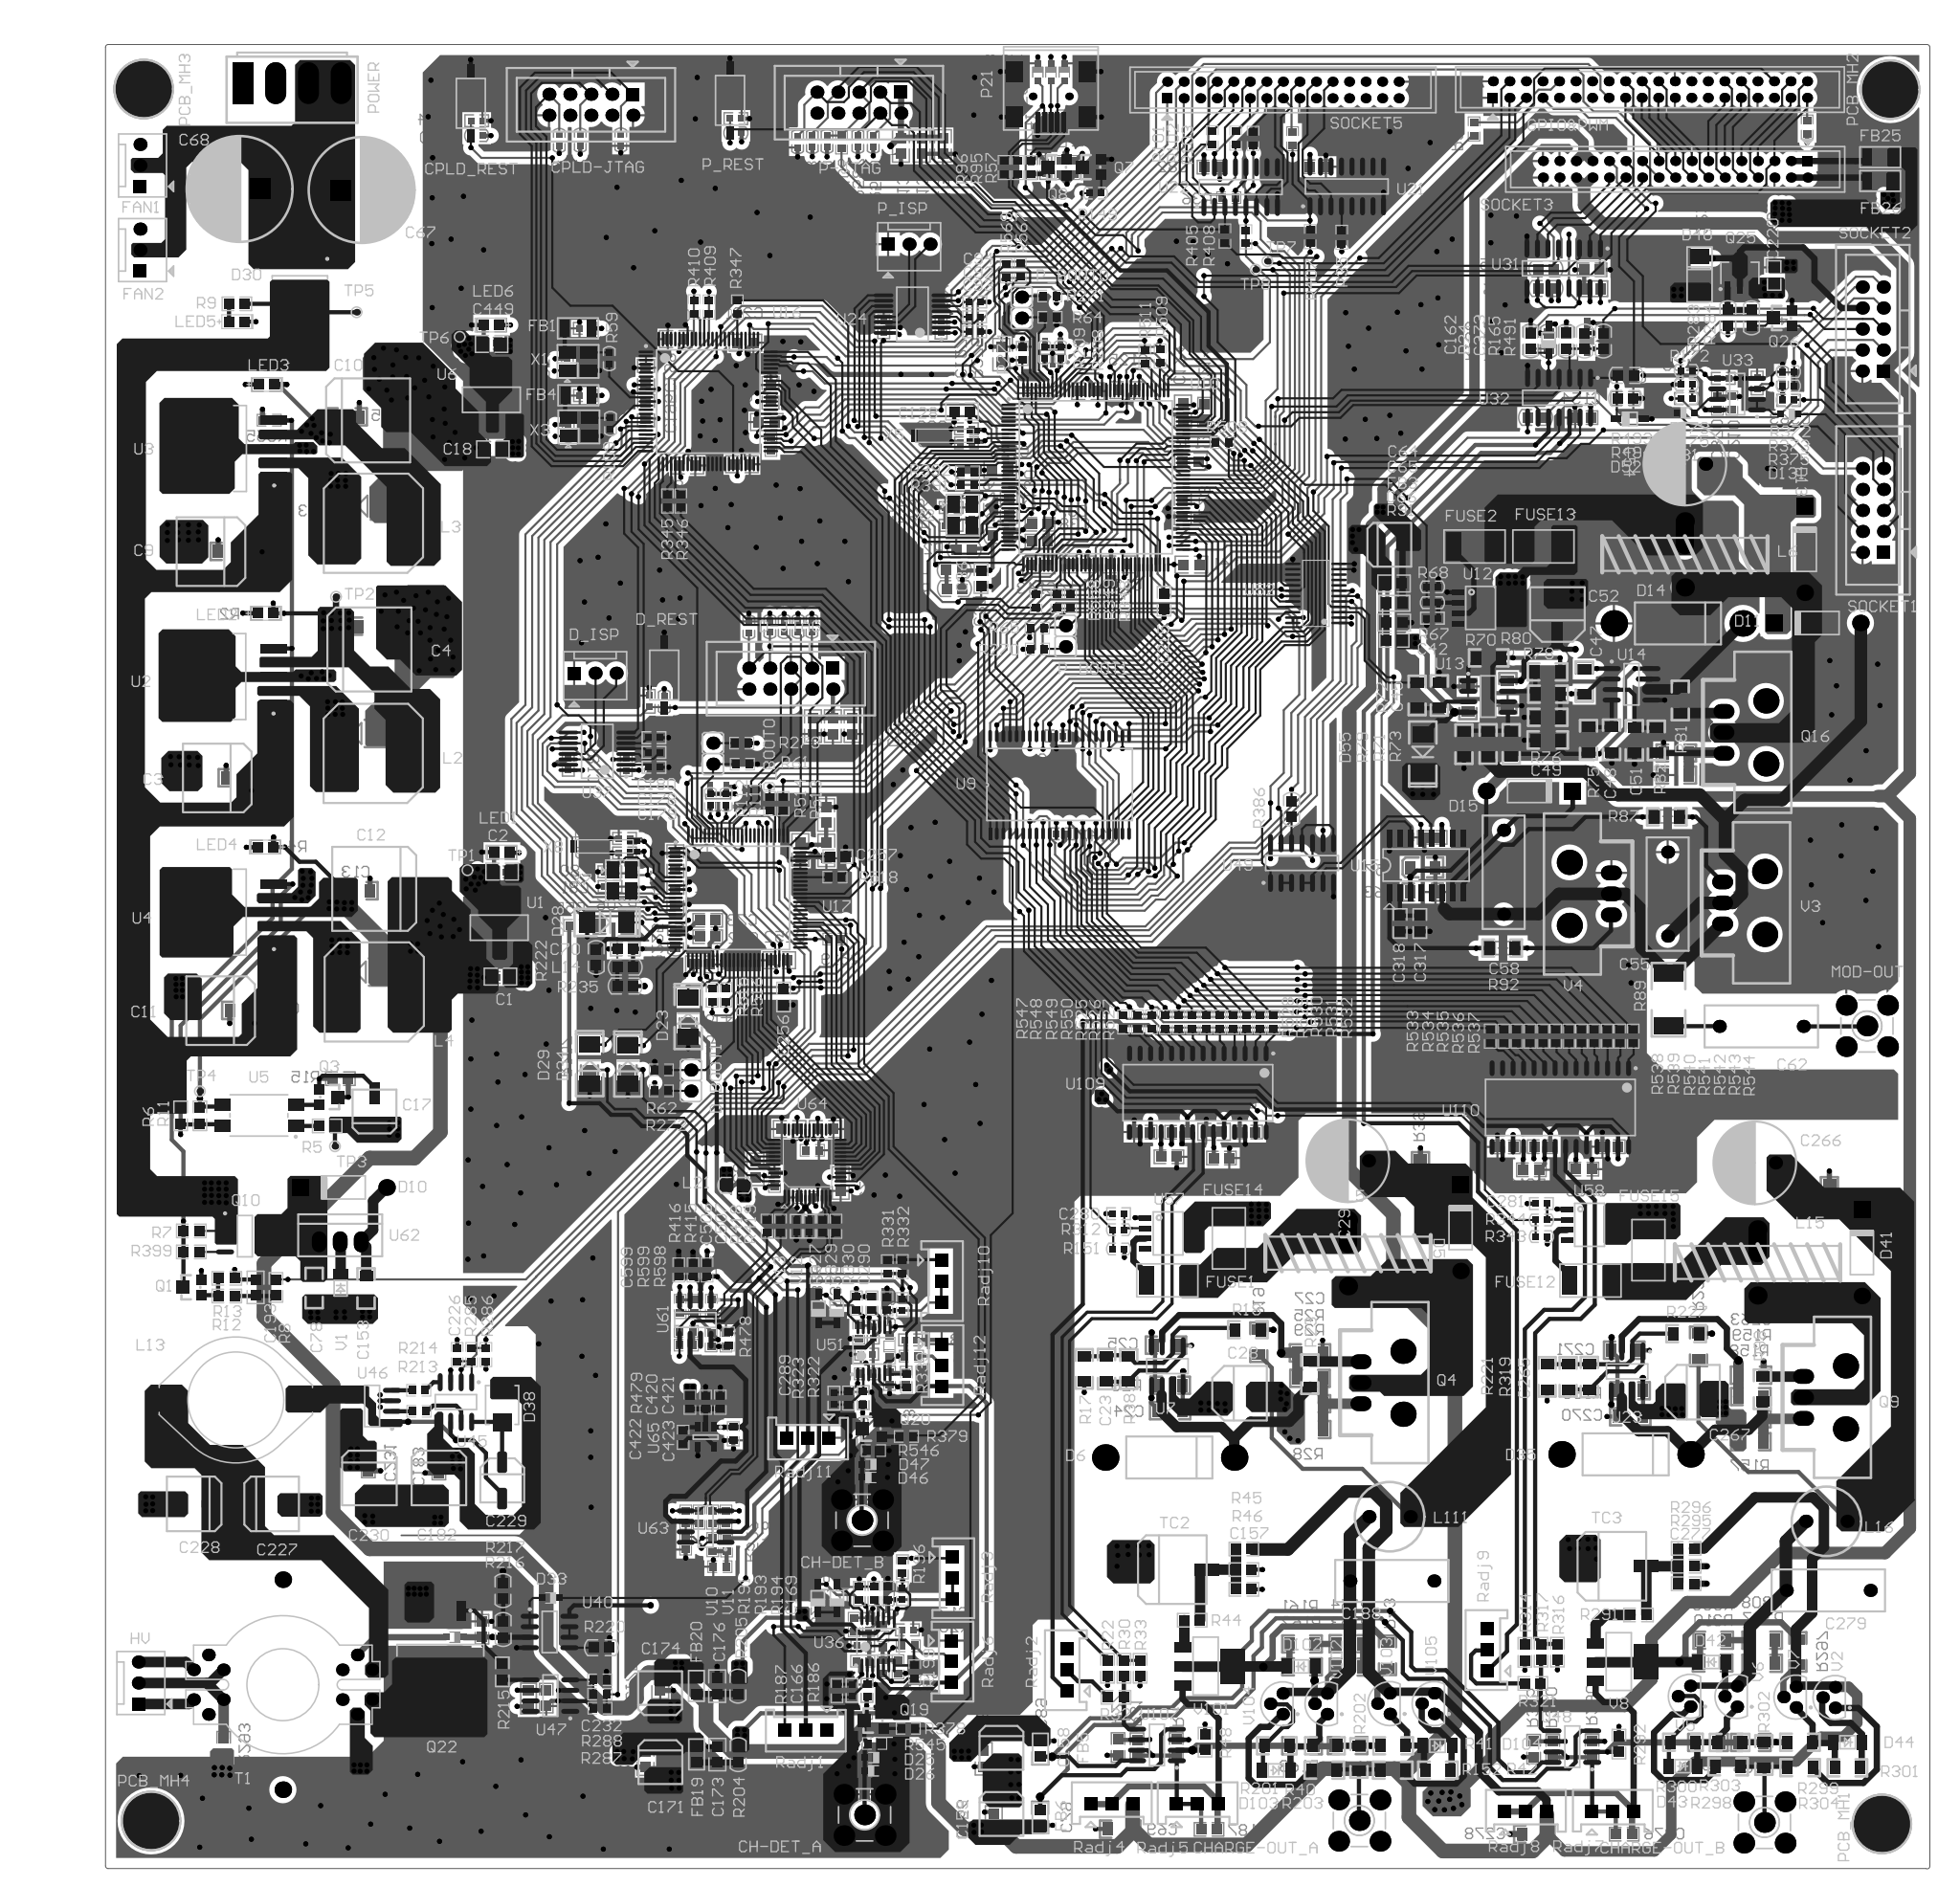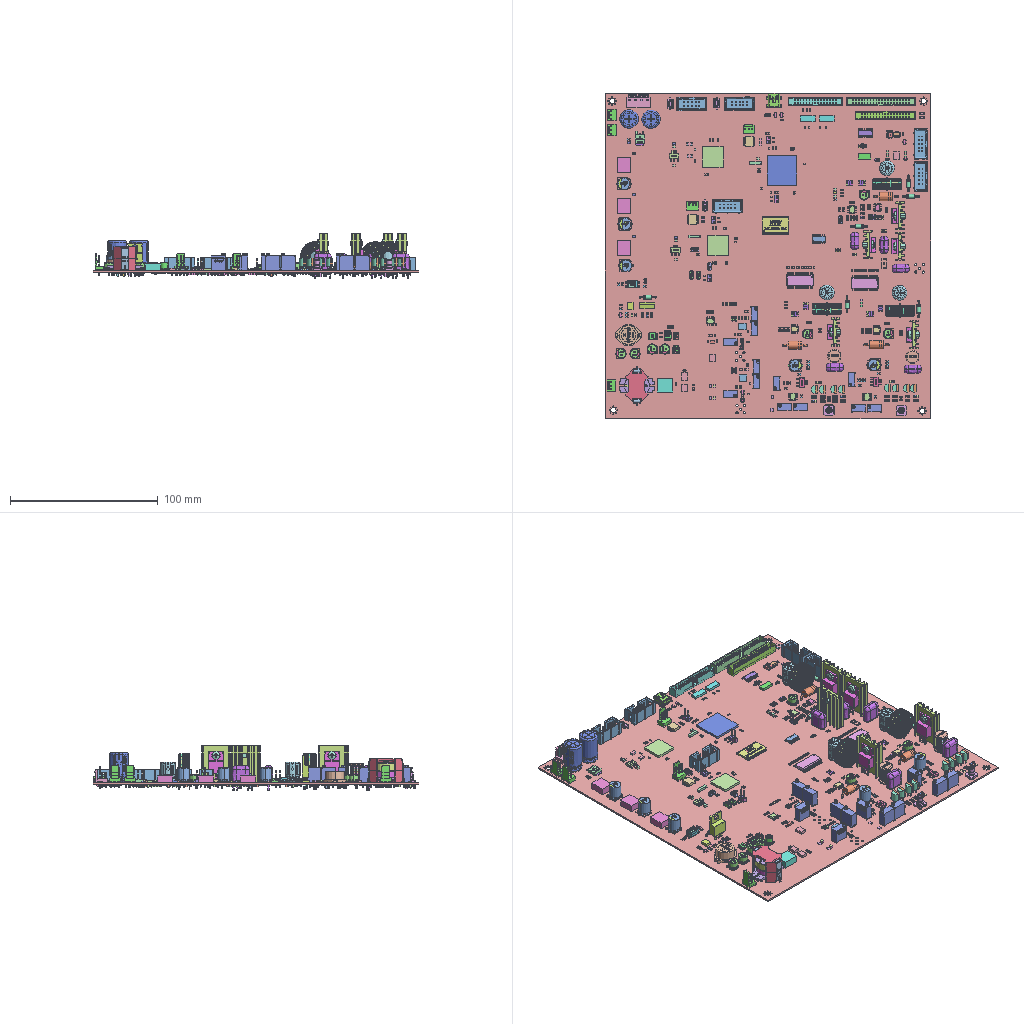Circuit board layout | Altium Designer | box 220.7 x 220.7 x 30 mm
Layer stack:
# Altium Designer layer stack of  (unit mm; dielectric type: 0 none, 1 core, 2 prepreg, 3 surface material)
index,name,kind,layer,copper_thickness_mm,dielectric_type,dielectric_thickness_mm,dielectric_material,dielectric_constant
0,Top Paste,other,,,,,,
1,Top Overlay,other,,,,,,
2,Top Solder,dielectric,,,3,0.0102,Solder Resist,3.5
3,Top Layer,copper,Top Layer,0.0356,,,,
4,Dielectric1,dielectric,,,1,0.32,FR-4,4.8
5,GND,copper,GND,0.0356,,,,
6,Dielectric5,dielectric,,,2,0.32,FR-4,4.8
7,POWER,copper,POWER,0.0356,,,,
8,Dielectric6,dielectric,,,1,0.32,FR-4,4.8
9,Bottom Layer,copper,Bottom Layer,0.0356,,,,
10,Bottom Solder,dielectric,,,3,0.0102,Solder Resist,3.5
11,Bottom Overlay,other,,,,,,
12,Bottom Paste,other,,,,,,
# drill layer pairs: low layer,high layer
drill_pair,Top Layer,Bottom Layer
Part placement, first 611 of 748 lines:
Designator,Comment,Layer,Footprint,Center-X(mm),Center-Y(mm),Rotation
R569,0R/NC,TopLayer,RES_0603,108.61,192.938,270
R567,0R/NC,TopLayer,RES_0603,110.312,193.015,270
R565,0R/NC,BottomLayer,RES_0603,73.05,105.334,90
R564,0R/NC,BottomLayer,RES_0603,74.752,105.359,90
R455,0R/NC,BottomLayer,RES_0603,80.162,171.958,270
R599,10K,TopLayer,RES_0603,70.739,72.085,270
R598,10K,TopLayer,RES_0603,72.441,72.085,90
R596,10K,BottomLayer,R0603,83.439,149.936,270
R595,10K,BottomLayer,R0603,77.495,149.835,270
R594,10K,BottomLayer,R0603,80.035,149.911,90
R593,10K,BottomLayer,R0603,81.763,149.936,90
R592,10K,BottomLayer,R0603,85.115,149.962,90
R591,10K,BottomLayer,R0603,83.388,208.559,90
R590,10K,BottomLayer,R0603,86.944,208.61,270
R589,10K,BottomLayer,R0603,92.532,208.61,270
R588,10K,BottomLayer,R0603,85.166,208.585,270
R587,10K,BottomLayer,R0603,90.678,208.61,270
R556,0R,BottomLayer,RES_0603,56.566,113.767,180
R207,1K,BottomLayer,R1206,58.217,97.815,90
R110,1K,BottomLayer,R1206,62.89,97.815,90
D34,1SMA4728A,TopLayer,DO-214AC,62.865,96.939,90
D29,1SMA4728A,TopLayer,DO-214AC,58.242,96.99,90
C599,0.1uF,TopLayer,CAP_0603,69.012,72.085,90
R558,0R,TopLayer,RES_0603,112.217,153.01,270
R555,0R/NC,BottomLayer,RES_0603,19.482,174.879,360
R550,0R,TopLayer,RES_0603,127.864,102.083,90
R549,0R,TopLayer,RES_0603,126.187,102.083,90
R548,0R,TopLayer,RES_0603,124.511,102.083,90
R547,0R,TopLayer,RES_0603,122.809,102.083,90
R546,1M/NC,TopLayer,RES_0603,92.558,50.241,180
R545,1M/NC,TopLayer,RES_0603,92.71,14.808,180
R544,0R,TopLayer,RES_0603,184.455,100.368,90
R543,0R,TopLayer,RES_0603,182.855,100.368,90
R542,0R,TopLayer,RES_0603,181.305,100.368,90
R541,0R,TopLayer,RES_0603,179.756,100.368,90
R540,0R,TopLayer,RES_0603,178.206,100.368,90
R539,0R,TopLayer,RES_0603,176.657,100.368,90
R538,0R,TopLayer,RES_0603,175.082,100.368,90
R537,0R,TopLayer,RES_0603,173.533,100.368,90
R536,0R,TopLayer,RES_0603,171.983,100.368,90
R535,0R,TopLayer,RES_0603,170.383,100.368,90
R534,0R,TopLayer,RES_0603,168.783,100.368,90
R533,0R,TopLayer,RES_0603,167.157,100.368,90
R532,0R,TopLayer,RES_0603,140.97,102.083,90
R531,0R,TopLayer,RES_0603,139.319,102.083,90
R530,0R,TopLayer,RES_0603,137.693,102.083,90
R529,0R,TopLayer,RES_0603,136.042,102.083,90
R528,0R,TopLayer,RES_0603,134.442,102.083,90
R527,0R,TopLayer,RES_0603,132.791,102.083,90
R526,0R,TopLayer,RES_0603,131.14,102.083,90
R525,0R,TopLayer,RES_0603,129.489,102.083,90
R496,1K,TopLayer,R0805,183.515,177.521,180
R495,1K,BottomLayer,R0805,176.378,184.455,270
R493,680R,TopLayer,R0805,183.591,180.289,180
R491,680R,TopLayer,R0805,180.848,184.455,270
D54,4.7V,BottomLayer,SOD-123,178.841,184.988,270
D52,4.7V,TopLayer,SOD-123,184.048,175.031,180
C449,22uF,TopLayer,C0805,46.38,184.099,180
C374,0.1uF,BottomLayer,CAP_0805,183.515,177.52,180
U64,AD9288BST100,TopLayer,LQFP48A,84.582,85.065,90
U16,EPM240GT100C5N,TopLayer,TQFP100_N,72.593,177.14,270
U17,STM32F407VGT6,TopLayer,LQFP100_N,76.175,117.094,0
Q20,NPN/CJ2302,TopLayer,SOT-23-3,92.405,52.883,180
Q19,NPN/CJ2302,TopLayer,SOT-23-3,92.634,17.577,180
Q7,NPN/SS8050LT1,TopLayer,SOT-23-3,118.974,205.486,180
C507,Cap Semi,TopLayer,C0603,84.836,77.368,270
C506,Cap Semi,TopLayer,C0603,83.236,77.368,270
C153,0.1uF,TopLayer,c1206,31.217,69.85,270
C78,0.33uF,TopLayer,c1206,24.943,69.901,270
C53,0.47uF,BottomLayer,c1206,164.49,141.148,90
C50,0.47uF,BottomLayer,c1206,169.266,141.859,270
C45,0.22uF,TopLayer,c1206,160.985,141.58,90
C1,22uF,TopLayer,C0805,47.447,107.569,360
C2,22uF,TopLayer,C0805,47.65,120.269,180
C3,220uF/35V,TopLayer,E8X10,2,13.198,131.597,180
C4,470uF/25V,TopLayer,E10X10.2,31.598,147.142,360
C5,0.1uF,BottomLayer,C1206,31.826,149.936,360
C6,0.1uF,BottomLayer,C0603,47.803,107.467,360
C7,0.1uF,BottomLayer,C0603,47.396,120.244,180
C8,0.1uF,BottomLayer,C1206,15.799,131.597,360
C9,220uF/35V,TopLayer,E8X10,2,12.436,158.979,180
C10,470uF/25V,TopLayer,E10X10.2,31.445,174.854,360
C11,220uF/35V,TopLayer,E8X10,2,13.605,103.454,180
C12,470uF/25V,TopLayer,E10X10.2,32.182,118.186,180
C13,0.1uF,BottomLayer,C1206,30.15,117.983,180
C14,0.1uF,BottomLayer,C1206,14.834,158.979,360
C15,0.1uF,BottomLayer,C1206,28.854,175.26,360
C16,0.1uF,BottomLayer,C1206,16.231,103.454,360
C17,47uF/16V,TopLayer,E5X5.4,32.233,91.278,90
C18,22uF,TopLayer,C0805,46.533,171.348,360
C19,0.1uF,BottomLayer,C0603,46.634,171.577,0
C20,0.1uF,BottomLayer,C0603,46.203,184.175,180
C23,47pF,TopLayer,C1206,120.777,60.096,270
C24,10nF,BottomLayer,C1206,128.448,55.093,180
C25,2.2nF,BottomLayer,C1206,127.94,62.967,360
C27,470pF,BottomLayer,C1206,145.364,62.027,360
C28,22uF/35V,TopLayer,E6.3X5.4,136.841,57.175,360
C29,2.2uF/450V,TopLayer,CAP-EL-10X13_5-5,149.936,85.293,360
C30,0.1uF,BottomLayer,CAP_0805,129.591,88.748,180
C31,0.1uF,BottomLayer,CAP_0805,137.821,88.773,180
C32,0.1uF,BottomLayer,CAP_0805,125.044,88.773,180
C33,0.1uF,BottomLayer,CAP_0805,134.645,85.623,180
C34,0.1uF,BottomLayer,C0603,57.709,185.979,360
C35,1uF,BottomLayer,CAP_0805,105.588,155.727,90
C36,0.1uF,TopLayer,CAP_0805,105.588,155.727,90
C37,1uF,BottomLayer,CAP_0805,112.7,162.28,180
C38,0.1uF,BottomLayer,CAP_0805,112.7,160.249,180
C39,0.1uF,BottomLayer,C0603,75.921,211.353,180
C40,20pF,BottomLayer,C0603,101.956,164.313,360
C41,20pF,BottomLayer,C0603,101.956,162.154,360
C42,470pF,TopLayer,C0603,160.172,150.927,360
C47,47pF,TopLayer,C1206,178.562,143.256,270
C48,2.2nF,TopLayer,C1206,181.864,136.22,270
C49,10nF,TopLayer,C1206,174.117,136.169,180
C51,470pF,TopLayer,C1206,184.607,136.144,270
C52,22uF/35V,TopLayer,E6.3X5.4,175.285,151.369,90
C54,2.2uF/450V,TopLayer,CAP-EL-10X13_5-5,190.703,169.57,360
C55,0.33uF/400V,TopLayer,CBB-400V-10mm,188.62,117.551,270
C56,0.1uF,BottomLayer,CAP_0805,160.147,124.409,180
C57,22uF/35V,BottomLayer,CAP_AVX-A,159.004,120.777,360
C58,0.1uF/400V,TopLayer,CBB-400V-10mm,168.783,120.193,90
C62,22nF/630V,TopLayer,CBB-400V-10mm,199.949,101.549,360
C63,0.1uF,BottomLayer,C1206,159.004,117.805,180
C64,10uF/25V,TopLayer,E5X5.4,154.981,159.791,360
C65,0.1uF,TopLayer,C0805,155.524,155.118,360
C66,0.1uF,TopLayer,C0805,155.55,150.393,180
C67,1000uF/35V,TopLayer,CAP-EL-12x20,30.658,202.717,360
C68,1000uF/35V,TopLayer,CAP-EL-12x20,15.9,202.844,180
C69,0.47uF,BottomLayer,C1206,122.403,4.47,180
C70,1uF,TopLayer,CAP_0805,62.535,110.922,360
C71,0.1uF,BottomLayer,CAP_0805,62.535,110.922,360
C72,1uF,BottomLayer,CAP_0805,72.517,112.395,180
C73,0.1uF,BottomLayer,CAP_0805,72.517,114.376,180
C74,0.1uF,BottomLayer,C0603,65.43,140.868,270
C75,0.1uF,BottomLayer,C0603,57.734,177.851,360
C79,0.1uF,BottomLayer,C0805,112.725,5.867,90
C80,20pF,BottomLayer,C0603,60.681,120.244,360
C81,20pF,BottomLayer,C0603,60.706,118.466,360
C82,0.1uF,BottomLayer,CAP_0805,133.502,205.486,180
C83,0.1uF,BottomLayer,CAP_0805,146.329,205.537,180
C84,10pF,BottomLayer,C0603,62.459,124.282,360
C85,10pF,BottomLayer,C0603,62.459,122.53,360
C86,100nF,BottomLayer,C0805,78.283,84.252,270
C87,100nF,BottomLayer,C0805,68.605,121.539,270
C88,100nF,BottomLayer,C0805,86.843,127.127,270
C89,0.1uF,BottomLayer,C0805,112.751,14.173,270
C90,0.1uF,BottomLayer,C0603,93.802,186.182,270
C91,0.1uF,BottomLayer,C0603,100.736,186.131,270
C92,0.1uF,TopLayer,C0603,104.8,187.376,360
C93,0.1uF,TopLayer,C0603,104.8,185.572,180
C94,0.1uF,TopLayer,C0603,104.826,189.179,180
C98,10pF,BottomLayer,C0603,103.81,173.838,360
C99,10pF,BottomLayer,C0603,103.81,172.136,360
C123,10uF,BottomLayer,C0805,129.972,164.186,90
C124,100nF,BottomLayer,C0805,129.997,175.946,90
C125,10uF,BottomLayer,C0805,123.165,178.511,180
C126,100nF,BottomLayer,C0805,118.516,178.384,180
C127,10uF,BottomLayer,C0805,108.026,182.804,270
C128,100nF,TopLayer,C0805,103.276,175.92,0
C129,10uF,BottomLayer,C0805,107.899,168.885,360
C130,100nF,BottomLayer,C0805,108.941,164.338,270
C131,10uF,BottomLayer,C0805,95.885,208.051,90
C132,100nF,BottomLayer,C0805,98.4,208.051,90
C133,10uF,BottomLayer,C0805,100.965,208.051,90
C134,100nF,BottomLayer,C0805,122.25,157.429,360
C141,10uF,BottomLayer,C0805,131.013,157.404,180
C142,100nF,BottomLayer,C0805,117.424,157.429,360
C143,10uF,BottomLayer,C0805,112.573,157.328,360
C146,100nF,BottomLayer,C0805,130.937,169.875,360
C147,100nF,BottomLayer,C0603,115.392,124.841,180
C148,100nF,BottomLayer,C0603,114.783,136.677,360
C151,0.1uF,BottomLayer,CAP_0805,179.476,193.065,180
C373,0.1uF,TopLayer,CAP_0805,176.352,184.48,270
C154,0.1uF,BottomLayer,CAP_0805,178.384,175.184,360
C155,100nF,BottomLayer,C0805,105.893,12.954,270
C156,100nF,BottomLayer,C0805,107.112,5.309,90
C157,0.1uF,TopLayer,CAP_0805,137.363,33.452,360
C158,10uF/25V,TopLayer,E5X5.4,108.026,14.259,270
C159,10uF/25V,TopLayer,E5X5.4,108.026,6.258,270
C162,0.1uF,TopLayer,CAP_0805,172.06,184.455,270
C163,0.47uF,BottomLayer,C0603,190.881,177.495,180
C164,330pF,BottomLayer,C0603,195.351,179.934,180
C165,470pF,BottomLayer,C0603,91.77,21.234,270
C166,1.5nF,TopLayer,C0603,89.967,21.234,270
C167,0.01uF,BottomLayer,C0603,91.262,26.619,180
C168,0.01uF,BottomLayer,C0603,91.973,29.21,270
C169,1.5nF,TopLayer,C0603,96.063,32.944,270
C170,0.22uF,BottomLayer,C0603,96.672,28.55,360
C171,10uF/25V,TopLayer,E5X5.4,66.777,12.532,270
C172,0.1uF,BottomLayer,C0805,64.999,12.903,90
C173,0.1uF,TopLayer,C0805,73.685,13.462,270
C174,10uF/25V,TopLayer,E5X5.4,66.777,20.92,90
C175,0.1uF,BottomLayer,C0805,66.777,22.174,90
C176,0.1uF,TopLayer,C0805,73.66,21.742,270
C177,0.1uF,BottomLayer,C0603,62.662,133.223,270
C178,0.1uF,TopLayer,C0603,66.015,134.696,360
C179,0.1uF,TopLayer,C0603,66.015,132.893,180
C180,0.1uF,TopLayer,C0603,66.015,136.474,180
C181,0.1uF,BottomLayer,C0603,55.651,133.248,270
C182,22uF/35V,TopLayer,CAP-ALU-6_3X5_4,40.005,46.928,270
C183,0.1uF,BottomLayer,CAP_0805,40.005,48.489,90
C184,0.1uF,BottomLayer,CAP_0805,45.212,28.626,270
C187,0.22nF,BottomLayer,CAP_0805,133.147,4.42,180
C188,0.33uF/400V,TopLayer,CBB-400V-10mm,155.27,34.468,180
C193,10uF,TopLayer,C0805,17.831,69.977,270
C195,10nF,BottomLayer,C0805,65.049,176.022,90
C196,100nF,BottomLayer,C0805,70.053,169.393,180
C197,10nF,BottomLayer,C0805,68.656,184.683,360
C198,100nF,BottomLayer,C0805,79.654,174.65,360
C199,10nF,BottomLayer,C0805,65.049,180.264,270
C200,100nF,BottomLayer,C0805,76.657,169.545,180
C201,10nF,BottomLayer,C0805,77.089,184.252,180
C202,100nF,BottomLayer,C0805,80.112,178.181,270
C210,0.1uF,BottomLayer,CAP_0603,196.393,176.936,270
C214,2.2uF,BottomLayer,CAP_0805,132.613,175.844,270
C215,2.2uF,TopLayer,CAP_0805,127.711,152.984,270
C220,10uF,TopLayer,CAP_0805,201.498,192.38,270
C221,10uF,BottomLayer,CAP_0805,192.684,193.497,90
C226,0.1uF,TopLayer,CAP_0603,42.215,61.849,270
C227,33uF/35V,TopLayer,CAP-ALU-6_3X5_4,19.772,43.79,360
C228,33uF/35V,TopLayer,CAP-ALU-6_3X5_4,10.403,43.79,180
C229,10uF/25V,TopLayer,CAP-ALU-5X5_4,47.65,46.634,90
C230,22uF/35V,TopLayer,CAP-ALU-6_3X5_4,31.598,46.928,270
C231,0.1uF,BottomLayer,CAP_0805,31.471,48.742,90
C232,0.01uF,TopLayer,CAP_0603,59.461,22.504,180
C233,0.1uF,BottomLayer,CAP_0805,52.984,20.294,90
C240,100pF,BottomLayer,C0603,113.411,205.435,270
C241,1uF,BottomLayer,C0603,111.684,205.435,270
C242,100nF,BottomLayer,C0805,90.043,137.871,90
C243,100nF,BottomLayer,C0805,86.766,89.129,180
C244,0.1uF,BottomLayer,C0603,44.577,211.099,180
C245,100nF,BottomLayer,C0805,68.605,117.145,90
C246,10uF,BottomLayer,C0805,133.756,88.798,360
C247,10uF,BottomLayer,C0805,83.718,122.885,90
C248,10uF,BottomLayer,C0805,201.549,192.405,270
C249,10uF,BottomLayer,C0805,85.242,137.871,90
C250,10uF,BottomLayer,C0805,88.595,82.601,90
C251,10uF,BottomLayer,C0805,71.806,109.042,180
C252,10uF,BottomLayer,C0805,81.178,109.55,360
C253,10uF,BottomLayer,C0805,86.868,122.834,90
C254,100nF,BottomLayer,C0805,82.423,89.129,360
C255,100nF,BottomLayer,C0805,87.655,137.871,90
C256,2.2uF,TopLayer,CAP_0805,81.686,105.105,270
C257,2.2uF,TopLayer,CAP_0805,88.24,122.098,360
C263,470pF,BottomLayer,C1206,198.704,59.334,360
C265,47pF,TopLayer,C1206,179.172,59.131,270
C266,2.2uF/450V,TopLayer,CAP-EL-10X13_5-5,199.161,85.039,360
C267,22uF/35V,TopLayer,E6.3X5.4,191.628,57.302,360
C270,10nF,BottomLayer,C1206,184.099,54.356,180
C271,2.2nF,BottomLayer,C1206,183.363,62.357,360
C276,0.22nF,BottomLayer,CAP_0805,183.363,3.835,180
C277,0.1uF,TopLayer,CAP_0805,190.856,34.138,360
C278,0.47uF,BottomLayer,C1206,172.491,3.861,180
C279,0.33uF/400V,TopLayer,CBB-400V-10mm,208.051,33.325,180
C280,470pF,TopLayer,C0603,122.212,78.892,360
C281,470pF,TopLayer,C0603,173.355,80.112,360
C282,0.1uF,BottomLayer,CAP_0805,173.457,86.995,180
C283,0.1uF,BottomLayer,CAP_0805,181.686,86.995,180
C284,0.1uF,BottomLayer,CAP_0805,168.986,86.969,180
C285,0.1uF,BottomLayer,CAP_0805,178.486,84.277,180
C288,470pF,BottomLayer,C0603,91.313,56.642,270
C289,1.5nF,TopLayer,C0603,87.782,56.591,270
C290,1.5nF,TopLayer,C0603,96.063,67.92,270
C291,0.01uF,BottomLayer,C0603,92.532,64.567,270
C292,0.01uF,BottomLayer,C0603,91.745,61.9,180
C293,0.22uF,BottomLayer,C0603,97.053,63.627,360
C311,39pF,BottomLayer,CAP_0603,69.926,64.668,360
C317,1uF,TopLayer,CAP_0805,158.648,113.995,270
C318,0.1uF,TopLayer,CAP_0805,156.261,113.995,270
C330,39pF,BottomLayer,CAP_0603,69.19,67.666,270
C363,0.47uF,BottomLayer,C0603,203.251,177.267,360
C364,330pF,BottomLayer,C0603,199.441,179.375,270
C370,0.1uF,BottomLayer,CAP_0603,194.64,176.936,270
C411,0.1uF,BottomLayer,CAP_0603,85.166,86.563,180
C412,0.1uF,BottomLayer,CAP_0603,80.594,82.931,270
C413,4.7uF,BottomLayer,CAP_0603,84.379,80.848,360
C420,100nF,TopLayer,CAP_0603,72.263,56.083,270
C421,10uF,TopLayer,CAP_0603,74.041,56.083,270
C422,10uF,TopLayer,CAP_0603,69.545,51.841,90
C423,10uF,TopLayer,CAP_0603,75.616,52.273,270
C424,100nF,BottomLayer,CAP_0603,75.616,52.273,90
C501,39pF,BottomLayer,CAP_0603,73.101,42.189,270
C502,39pF,BottomLayer,CAP_0603,71.476,42.189,270
CH-DET_A,SMB,TopLayer,SMB_V-RJ45,91.491,6.172,360
CH-DET_B,SMB,TopLayer,SMB_V-RJ45,91.186,41.808,360
CHARGE-OUT_A,SMB,TopLayer,SMB_V-RJ45,151.333,5.486,90
CHARGE-OUT_B,SMB,TopLayer,SMB_V-RJ45,200.33,5.258,90
CPLD-JTAG,IDC2X5-2_54,TopLayer,IDC2X5-2_54,58.395,213.03,180
CPLD_REST,SW,TopLayer,SW-6X3X2.5,43.866,213.208,270
D2,1N5822,BottomLayer,D1810,29.807,136.982,180
D3,1N5822,BottomLayer,D1810,30.544,164.49,180
D4,1N5822,BottomLayer,D1810,30.34,108.128,180
D5,UF4007,TopLayer,DO-41_-_10.46mm,163.576,77.191,90
D6,SB560,TopLayer,SB560,128.399,49.403,360
D10,1N4004,TopLayer,DO-41_-_10.46mm,28.448,82.067,180
D11,ZPY15,TopLayer,DO-41_-_10.46mm,206.705,150.343,180
D13,UF4007,TopLayer,DO-41_-_10.46mm,205.207,159.233,90
D14,SB560,TopLayer,DO-201AD,189.918,150.292,360
D15,UF4007,TopLayer,DO-41_-_10.46mm,171.907,130.023,360
D23,1SMA4728A,TopLayer,DO-214AC,70.155,102.68,90
D24,4.7V,TopLayer,SOD-123,174.219,184.582,270
D25,1N4148WS,TopLayer,SOD323,92.583,13.106,180
D26,1N4148WS,TopLayer,SOD323,92.583,11.506,360
D27,1N4148,BottomLayer,SOD-323,93.751,27.758,360
D28,1SMA4728A,TopLayer,DO-214AC,60.287,114.122,360
D30,50WQ03FN,TopLayer,TO-252AA,23.19,191.166,270
D31,1N4148WS,TopLayer,SOD323,190.83,175.768,360
D32,1N4148WS,BottomLayer,SOD323,41.935,27.661,180
D33,1N4148WS,TopLayer,SOD323,53.518,32.41,180
D35,SB560,TopLayer,SB560,183.593,49.784,360
D38,10BQ060,TopLayer,DO-214AA-L,47.65,55.753,270
D40,UF4007(US1M),TopLayer,DO-214AA,192.481,192.507,90
D41,UF4007,TopLayer,DO-41_-_10.46mm,212.115,74.168,90
D42,1N4148,TopLayer,DO-213AA,193.904,24.663,180
D43,1N4148,TopLayer,DO-213AA,190.449,12.065,360
D44,1N4148,TopLayer,DO-213AA,210.388,14.961,360
D45,1N4148,BottomLayer,DO-213AA,188.62,126.949,180
D46,1N4148WS,TopLayer,SOD323,92.253,46.99,360
D47,1N4148WS,TopLayer,SOD323,92.253,48.565,180
D48,1N4148,BottomLayer,SOD-323,94.513,62.835,360
D49,1N4148,BottomLayer,DO-213AA,168.707,111.023,180
D55,IN4001/M1,TopLayer,DO-214AC,159.004,134.556,270
D102,1N4148,TopLayer,DO-213AA,144.272,24.13,180
D103,1N4148,TopLayer,DO-213AA,141.249,11.557,360
D104,1N4148,TopLayer,DO-213AA,160.782,14.529,360
D131,1N4148WS,TopLayer,SOD323,203.327,175.59,180
D-JTAG,IDC2X5-2_54,TopLayer,IDC2X5-2_54,82.575,143.612,180
D_BOOT0,PLS-2,TopLayer,PLS-2-2_54,73.152,134.544,270
D_BOOT1,PLS-2,TopLayer,PLS-2-2_54,70.485,94.996,90
D_ISP,KF2510-3A,TopLayer,KF2510-3A,58.903,144.272,360
D_REST,SW,TopLayer,SW-6X3X2.5,67.259,144.043,90
ESD23,PESD5V0S1BA,BottomLayer,SOD323,112.446,216.967,270
ESD24,PESD5V0S1BA,BottomLayer,SOD323,115.646,216.967,270
ESD25,PESD5V0S1BA,BottomLayer,SOD323,114.021,216.967,270
FAN1,KF2510-3A,TopLayer,KF2510-3A,3.861,205.689,90
FAN2,KF2510-3A,TopLayer,KF2510-3A,3.861,195.453,90
FB1,60,TopLayer,SMD1206-L,56.82,185.979,180
FB3,60,TopLayer,SMD0805-L,155.575,152.73,180
FB4,60,TopLayer,SMD1206-L,56.871,177.876,180
FB5,60,TopLayer,SMD0805-L,112.751,14.173,270
FB6,60,TopLayer,SMD0805-L,112.725,5.791,90
FB18,60,BottomLayer,SMD0805-L,179.502,190.779,180
FB19,60,TopLayer,SMD0805-L,71.171,13.487,270
FB20,60,TopLayer,SMD0805-L,71.145,21.768,270
FB25,60,TopLayer,SMD1206-L,214.325,206.68,180
FB26,60,TopLayer,SMD1206-L,214.325,203.81,180
FB27,60,BottomLayer,SMD0805-L,50.851,20.244,270
FUSE1,ASMD050-1812(30V,0.5A),TopLayer,SMD1812-Fuse,128.092,70.815,360
FUSE2,ASMD050-1812(30V,0.5A),TopLayer,SMD1812-Fuse,165.252,159.588,360
FUSE12,ASMD050-1812(30V,0.5A),TopLayer,SMD1812-Fuse,179.273,70.79,360
FUSE13,ASMD050-1812(30V,0.5A),TopLayer,SMD1812-Fuse,173.609,159.614,180
FUSE14,ASMD050-1812(30V,0.5A),TopLayer,SMD1812-Fuse,135.534,75.921,270
FUSE15,ASMD050-1812(30V,0.5A),TopLayer,SMD1812-Fuse,186.284,74.498,270
GPIO&PWM,HEAD2X20-2MM-A,TopLayer,IDC2X20-2.0mm-A,186.488,214.868,360
HV,KF2510-3A,TopLayer,KF2510-3A,3.658,22.123,90
L2,68uH,TopLayer,L330,32.059,134.569,0
L3,68uH,TopLayer,L330,32.084,162.408,0
L4,68uH,TopLayer,L330,32.186,105.715,0
L5,200uH,TopLayer,L200/1.4A,149.962,74.117,90
L6,200uH,TopLayer,L200/1.4A,190.703,158.648,90
L11,600R,100MHz,BottomLayer,R0805,102.337,156.769,360
L13,330uH,TopLayer,PBS5022,15.443,56.363,180
L14,600R,100MHz,TopLayer,R0805,62.535,108.712,360
L15,200uH,TopLayer,L200/1.4A,199.492,73,90
L16,330uH,TopLayer,L-9x12,207.823,41.681,180
L21,600R,100MHz,TopLayer,R0805,75.794,82.321,180
L111,330uH,TopLayer,L-9x12,154.991,42.24,180
LED1,LED,TopLayer,LED_0805,47.65,122.631,180
LED2,LED,TopLayer,LED_0805,19.025,151.511,360
LED3,LED,TopLayer,LED_0805,19.126,179.197,360
LED4,LED,TopLayer,LED_0805,19.05,123.241,180
LED5,LED,TopLayer,LED_0805,15.545,186.792,360
LED6,LED,TopLayer,LED_0805,46.33,186.385,180
MOD-OUT,SMB,TopLayer,SMB_V-RJ45,212.725,101.6,90
P21,MiniUSB,TopLayer,MiniUSB-A,114.021,213.996,270
P-JTAG,IDC2X5-2_54,TopLayer,IDC2X5-2_54,90.805,213.284,180
P_BOOT0,PLS-2,TopLayer,PLS-2-2_54,110.49,188.493,270
P_BOOT1,PLS-2,TopLayer,PLS-2-2_54,115.799,148.742,90
P_ISP,KF2510-3A,TopLayer,KF2510-3A,96.876,196.164,360
P_REST,SW,TopLayer,SW-6X3X2.5,75.214,213.563,90
PCB_MH1,MOUNTING HOLE 3MM,TopLayer,MOUNTING_HOLE_3MM,214.528,5.08,90
PCB_MH2,MOUNTING HOLE 3MM,TopLayer,MOUNTING_HOLE_3MM,215.519,214.859,90
PCB_MH3,MOUNTING HOLE 3MM,TopLayer,MOUNTING_HOLE_3MM,4.293,214.935,90
PCB_MH4,MOUNTING HOLE 3MM,TopLayer,MOUNTING_HOLE_3MM,5.182,5.436,90
POWER,HEAD4-3.96A,TopLayer,VH-3_96-4,22.247,215.646,360
Q1,S9013LT1,TopLayer,SOT-23,10.135,69.99,180
Q3,S9012LT1,TopLayer,SOT-23,26.67,93.002,360
Q4,IRF740,TopLayer,TO220V1,154.076,58.445,360
Q8,SI2301CDS-T1-GE3,TopLayer,SOT-23,114.833,205.473,180
Q9,IRF740,TopLayer,TO220V1,207.594,56.667,360
Q16,IRF740,TopLayer,TO220V1,197.968,137.109,0
Q25,2SA1416,TopLayer,SOT89,197.358,192.234,90
Q26,MMBF170,TopLayer,SOT-23,202.514,187.236,180
R1,270R,BottomLayer,RES_0805,47.625,122.555,360
R2,1K,BottomLayer,RES_0805,19.05,151.511,180
R3,470R,BottomLayer,RES_0805,19.152,179.197,180
R4,1K,BottomLayer,RES_0805,19.05,123.241,180
R5,100R,TopLayer,RES_0805,26.492,89.51,180
R6,47K,TopLayer,RES_0805,8.763,90.729,90
R7,47K,TopLayer,RES_0805,10.058,76.81,360
R8,1K,TopLayer,RES_0805,20.295,69.977,270
R9,20K,TopLayer,RES_0805,15.57,188.951,360
R11,47K,TopLayer,RES_0805,11.1,90.729,270
R12,2.2K,TopLayer,RES_0805,14.351,68.936,180
R13,2.2K,TopLayer,RES_0805,14.351,71.069,360
R15,100K,BottomLayer,RES_0805,28.092,95.225,360
R16,270R,BottomLayer,RES_0805,46.38,186.385,360
R17,1K8,TopLayer,R1206,118.059,60.122,90
R18,150K,TopLayer,R1206,137.846,64.872,360
R19,56K,BottomLayer,R1206,139.167,63.348,270
R22,50R,TopLayer,RES_0805,120.879,23.901,270
R23,22R,TopLayer,R1206,145.339,59.487,90
R25,1K,BottomLayer,R1206,145.364,58.979,360
R26,8K2,BottomLayer,R1206,128.448,58.141,180
R27,510R,BottomLayer,RES_0805,122.149,14.326,90
R28,4R7,BottomLayer,R1206,145.44,52.781,360
R29,2R2,BottomLayer,R1206,145.415,55.905,360
R30,20R,TopLayer,RES_0805,122.86,23.901,270
R31,2.7K,BottomLayer,RES_0805,124.435,14.3,270
R32,100R,TopLayer,RES_0805,121.895,20.396,360
R33,50R,TopLayer,RES_0805,124.816,23.901,90
R34,2K,BottomLayer,RES_0805,128.295,85.776,360
R35,0R,TopLayer,RES_0603,149.2,197.002,270
R36,0R,BottomLayer,RES_0603,135.534,201.803,180
R38,1M,TopLayer,R1206,123.444,60.096,90
R39,1M,BottomLayer,R1206,158.725,83.947,270
R40,1K5,TopLayer,R1206,147.168,14.529,360
R41,1K5,TopLayer,R1206,155.423,14.529,360
R42,390R,TopLayer,R1206,160.833,11.582,360
R43,1K,BottomLayer,R1206,154.737,25.476,90
R44,470R,TopLayer,RES_0805,131.115,29.718,360
R45,2K7,TopLayer,RES_0805,137.363,38.329,180
R46,2K7,TopLayer,RES_0805,137.363,35.839,360
R47,50R,BottomLayer,RES_0805,129.184,14.326,90
R48,3K3,TopLayer,RES_0805,132.664,14.961,270
R57,0R,TopLayer,RES_0603,111.608,205.435,270
R58,10K,BottomLayer,R0603,55.55,181.61,90
R59,22R,TopLayer,R0603,60.604,182.321,90
R61,10K,TopLayer,RES_0603,76.708,133.274,360
R62,10K,TopLayer,RES_0603,66.904,96.291,180
R63,10K,BottomLayer,R0603,75.921,209.626,180
R64,10K,TopLayer,RES_0603,113.919,187.325,360
R65,10K,TopLayer,RES_0603,112.37,149.733,180
R66,1M,BottomLayer,R0603,104.419,163.576,270
R67,10K,TopLayer,R0603,160.172,152.806,180
R68,10K,TopLayer,R0603,160.172,154.711,180
R70,20K,TopLayer,R1206,166.98,146.126,360
R71,1M,TopLayer,R1206,166.903,135.712,90
R72,10K,TopLayer,R1206,158.318,141.58,90
R73,20K,TopLayer,R1206,169.697,135.712,90
R74,1M,BottomLayer,R1206,201.117,165.989,270
R75,8K2,TopLayer,R1206,179.045,136.22,90
R76,22K,TopLayer,R1206,174.117,138.938,360
R77,150K,BottomLayer,R1206,178.537,143.256,90
R78,22K,TopLayer,R1206,174.142,141.732,360
R79,20K,TopLayer,R1206,163.982,135.687,90
R80,20K,TopLayer,R1206,174.092,144.424,180
R81,22R,TopLayer,R1206,190.144,140.97,270
R82,1K,TopLayer,R1206,187.249,136.144,270
R84,2R2,BottomLayer,R1206,189.662,131.953,360
R85,2R2,BottomLayer,R1206,189.662,134.62,360
R87,220R,TopLayer,R1206,188.519,126.898,180
R89,100R,TopLayer,RES_2512,188.722,104.775,270
R91,10R,TopLayer,RES_0805,155.55,148.234,0
R92,220R,TopLayer,R1206,168.605,111.023,180
R95,0R,TopLayer,RES_0603,109.982,205.435,270
R96,0R,TopLayer,RES_0603,108.356,205.435,270
R98,22R,TopLayer,R1206,200.076,57.658,90
R100,10K,BottomLayer,R0603,44.577,209.296,180
R101,0R/NC,TopLayer,RES_0603,133.553,209.017,90
R102,0R/NC,TopLayer,RES_0603,136.373,208.991,90
R103,0R/NC,TopLayer,RES_0603,138.481,208.966,90
R104,0R/NC,BottomLayer,RES_0603,143.256,208.915,90
R106,1K,BottomLayer,R1206,70.155,103.505,90
R108,10K,BottomLayer,R0603,55.651,173.634,90
R109,22R,TopLayer,R0603,60.757,174.473,90
R111,4.7K,TopLayer,R0603,74.752,128.981,270
R112,4.7K,TopLayer,R0603,72.847,128.981,270
R113,10K,BottomLayer,R0603,67.259,140.818,270
R114,1M,BottomLayer,R0603,63.271,119.151,270
R149,4.7K,TopLayer,R0603,119.405,202.336,360
R150,47K,BottomLayer,RES_0603,115.189,205.435,90
R151,10K,TopLayer,R0603,122.212,74.625,180
R152,100R,TopLayer,R1206,155.372,11.582,360
R153,12K,BottomLayer,R1206,150.139,24.054,180
R154,12K,BottomLayer,R1206,150.114,26.873,360
R155,0R/NC,BottomLayer,R0805,173.888,193.167,180
R156,0R,BottomLayer,R0805,173.888,190.805,360
R157,4R7,BottomLayer,R1206,198.679,51.308,360
R158,2R2,BottomLayer,R1206,198.679,54.077,360
R159,1K,BottomLayer,R1206,198.679,56.769,360
R160,8K2,BottomLayer,R1206,184.074,57.48,180
R161,12K,BottomLayer,R1206,144.399,26.848,360
R162,12K,BottomLayer,R1206,144.399,24.079,180
R163,150K,BottomLayer,R1206,144.399,14.529,180
R164,1.8K,BottomLayer,R1206,149.911,14.554,180
R165,10K,TopLayer,R0805,178.562,184.455,90
R166,680R,BottomLayer,R0805,172.06,184.48,270
R168,1K,BottomLayer,R0805,174.219,184.455,270
R172,330K,TopLayer,R0603,190.881,180.899,180
R173,1M,TopLayer,R0603,190.881,179.197,180
R174,330K,BottomLayer,R0603,190.881,179.197,180
R175,0ohm,TopLayer,R0603,190.881,177.495,360
R186,10K,TopLayer,RES_0603,91.796,21.234,90
R187,200K,TopLayer,RES_0603,88.138,21.209,90
R188,6.8K,BottomLayer,RES_0603,91.262,24.765,360
R189,6.8K,BottomLayer,RES_0603,92.608,32.944,90
R190,18K,BottomLayer,RES_0603,90.856,32.944,270
R191,27K,TopLayer,RES_0603,90.856,32.944,90
R192,15K,BottomLayer,RES_0603,90.221,29.21,90
R193,3.9K,TopLayer,RES_0603,92.634,32.944,90
R194,1.5K,TopLayer,RES_0603,94.31,32.969,270
R195,27K,BottomLayer,RES_0603,96.063,36.17,270
R196,30K,TopLayer,RES_0603,96.063,36.17,270
R197,15K,BottomLayer,RES_0603,95.529,24.079,90
R198,1K,BottomLayer,RES_0603,93.751,24.079,270
R199,100K,TopLayer,RES_0603,97.561,23.47,90
R200,10K,BottomLayer,RES_0603,96.774,26.619,360
R201,390R,TopLayer,R1206,141.351,14.529,180
R202,2K2,TopLayer,R1206,151.282,13.056,270
R203,100R,TopLayer,R1206,147.091,11.582,360
R204,100R,TopLayer,R0805,76.2,13.462,90
R205,100R,TopLayer,R0805,76.175,21.742,90
R206,1K,BottomLayer,R1206,61.112,113.767,360
R208,4.7K,TopLayer,R0603,115.189,183.083,270
R209,4.7K,TopLayer,R0603,113.259,183.083,270
R212,100R,BottomLayer,R0805,172.644,175.209,360
R213,33R,TopLayer,RES_0603,37.592,54.991,360
R214,33R,TopLayer,RES_0603,37.567,57.531,360
R215,33R,TopLayer,RES_0805,47.676,23.47,270
R216,150K,TopLayer,R0805,47.777,28.6,270
R217,100K,TopLayer,R0805,47.752,33.299,90
R220,1K,TopLayer,R0805,59.665,26.391,360
R221,1K8,TopLayer,R1206,174.041,59.157,90
R222,0R,TopLayer,R0805,59.03,109.88,270
R225,47R,BottomLayer,R0805,68.631,112.116,90
R226,1K,BottomLayer,RES_0603,116.815,205.435,90
R227,150K,TopLayer,R1206,190.856,64.389,360
R232,10K,BottomLayer,R0603,57.099,208.737,270
R234,10K,BottomLayer,R0603,54.559,208.712,270
R235,0R,TopLayer,R0805,62.535,106.426,180
R236,56K,BottomLayer,R1206,192.354,62.84,270
R269,0R,BottomLayer,R0805,103.53,159.22,180
R270,1K,TopLayer,RES_0603,112.395,147.193,180
R271,1K,TopLayer,RES_0603,113.894,189.89,360
R272,1K,TopLayer,RES_0603,66.904,93.751,180
R273,1K,TopLayer,RES_0603,76.632,135.814,360
R274,0R,TopLayer,RES_0603,110.566,182.944,90
R275,0R/NC,BottomLayer,RES_0603,110.566,182.956,270
R276,47R,BottomLayer,R0805,107.925,160.934,360
R277,0R,BottomLayer,R0805,102.362,154.508,180
R283,4.7K,TopLayer,R0805,195.91,187.274,270
R284,560R,TopLayer,R0805,198.755,187.249,90
R285,100R,TopLayer,RES_0603,43.967,61.849,270
R286,10K,TopLayer,RES_0603,45.695,61.849,90
R287,10K,TopLayer,RES_0603,59.487,19.075,360
R288,100R,TopLayer,RES_0603,59.461,20.777,180
R290,50R,BottomLayer,RES_0805,179.476,14.122,90
R291,470R,TopLayer,RES_0805,185.09,30.353,360
R292,3K3,TopLayer,RES_0805,182.728,14.732,270
R293,0R,BottomLayer,RES_0805,13.97,14.478,270
R294,10K,BottomLayer,R0603,62.001,208.763,90
R295,2K7,TopLayer,RES_0805,190.856,36.246,360
R296,2K7,TopLayer,RES_0805,190.856,38.405,180
R297,1K,BottomLayer,R1206,204.368,25.883,90
R298,1K5,TopLayer,R1206,196.113,14.935,360
R299,1K5,TopLayer,R1206,204.622,14.961,360
R300,390R,TopLayer,R1206,190.475,14.961,180
R301,390R,TopLayer,R1206,210.363,11.862,360
R302,2K2,TopLayer,R1206,200.254,13.411,270
R303,100R,TopLayer,R1206,195.936,11.989,360
R304,100R,TopLayer,R1206,204.648,11.887,360
R305,150K,BottomLayer,R1206,193.497,14.935,180
R306,1.8K,BottomLayer,R1206,198.679,14.935,180
R307,12K,BottomLayer,R1206,200.05,24.511,180
R308,12K,BottomLayer,R1206,200.05,27.305,360
R309,12K,BottomLayer,R1206,194.132,27.305,360
R310,12K,BottomLayer,R1206,194.056,24.536,180
R312,10K,TopLayer,R0603,122.212,76.962,180
R313,1M,BottomLayer,R1206,208.178,80.924,270
R314,50R,TopLayer,RES_0805,171.348,25.832,270
R315,510R,BottomLayer,RES_0805,172.415,14.122,90
R316,50R,TopLayer,RES_0805,175.285,25.857,90
R317,20R,TopLayer,RES_0805,173.304,25.857,270
R318,2K,BottomLayer,RES_0805,172.136,84.201,360
R319,1M,TopLayer,R1206,176.581,59.157,90
R320,2.7K,BottomLayer,RES_0805,174.727,14.097,270
R321,100R,TopLayer,RES_0805,172.314,22.073,360
R322,10K,TopLayer,RES_0603,91.313,56.617,90
R323,200K,TopLayer,RES_0603,89.56,56.591,90
R324,6.8K,BottomLayer,RES_0603,91.719,59.512,360
R325,6.8K,BottomLayer,RES_0603,92.38,68.072,90
R326,18K,BottomLayer,RES_0603,90.5,68.072,270
R327,27K,TopLayer,RES_0603,90.5,68.072,90
R328,15K,BottomLayer,RES_0603,90.78,64.567,90
R329,3.9K,TopLayer,RES_0603,92.354,68.072,90
R330,1.5K,TopLayer,RES_0603,94.209,67.996,270
R332,30K,TopLayer,RES_0603,96.063,72.492,270
R333,15K,BottomLayer,RES_0603,94.513,58.979,90
R334,1K,BottomLayer,RES_0603,96.52,58.979,270
R336,10K,BottomLayer,RES_0603,97.155,61.671,360
R339,100K,TopLayer,RES_0603,96.571,58.649,90
R343,10K,TopLayer,R0603,173.355,76.124,180
R344,10K,TopLayer,R0603,173.355,78.13,180
R345,0R,TopLayer,RES_0603,67.64,165.1,270
R346,0R,TopLayer,RES_0603,69.266,165.1,270
R347,0R,TopLayer,RES_0603,76.098,188.57,90
R348,0R/NC,TopLayer,RES_0603,116.408,153.035,270
R349,0R/NC,TopLayer,RES_0603,114.732,153.035,270
R358,0R,BottomLayer,RES_0603,165.202,210.109,270
Pad and via stacks, first 82 of 139 lines:
# Altium Designer via and pad stacks of  (unit mm). Each distinct definition once, with the count of objects using it.
# via: kind,start_layer,end_layer,hole_mm,diameter_mm,mode(0 simple;1 top-mid-bottom;2 full stack),diameter_per_layer,count,example_net
# pad: kind,layer,hole_mm,hole_type(0 round;1 square;2 slot),plating,top_size,top_shape(1 round;2 rect;3 octagon;9 rounded rect),mid_size,bottom_size,mode,footprint,size_per_layer,count,example
pad,Top Layer,0,0,plated,0.9x1,2,0.9x1,0.9x1,0,RES_0603,,192,R567.2
pad,Top Layer,0,0,plated,1.27x1.27,2,1.27x1.27,1.27x1.27,0,RES_0805,,54,R48.1
pad,Top Layer,0,0,plated,0.8x0.8,2,0.8x0.8,0.8x0.8,0,C0603,,30,C169.1
pad,Top Layer,0,0,plated,2x1.1,2,2x1.1,2x1.1,0,SMD1206-L,,8,FB26.1
pad,Top Layer,0,0,plated,1.905x2.54,2,1.905x2.54,1.905x2.54,0,DO-214AC,,10,D29.2
pad,Top Layer,0,0,plated,0.9x1,2,0.9x1,0.9x1,0,CAP_0603,,14,C599.1
pad,Top Layer,0,0,plated,1.27x1.27,2,1.27x1.27,1.27x1.27,0,R0805,,32,R217.2
pad,Top Layer,0,0,plated,1.27x1.27,2,1.27x1.27,1.27x1.27,0,CAP_0805,,24,C36.1
pad,Top Layer,0,0,plated,1.27x1.524,2,1.27x1.524,1.27x1.524,0,C1206,,18,C48.2
pad,Top Layer,0,0,plated,1.27x1.27,2,1.27x1.27,1.27x1.27,0,C0805,,20,C18.1
pad,Top Layer,0,0,plated,1.2x0.8,2,1.2x0.8,1.2x0.8,0,SOD-123,,12,D52.2
pad,Top Layer,0,0,plated,1.2x2,2,1.2x2,1.2x2,0,SOT223,,12,U6.3
pad,Top Layer,0,0,plated,4.2x3,2,4.2x3,4.2x3,0,SOT223,,4,U6.4
pad,Top Layer,0,0,plated,0.6x2.2,1,0.6x2.2,0.6x2.2,0,SO8_N,,24,U63.5
pad,Top Layer,0,0,plated,0.6096x2.032,2,0.6096x2.032,0.6096x2.032,0,SOIC-16,,16,U15.5
pad,Top Layer,0,0,plated,0.6x2.2,1,0.6x2.2,0.6x2.2,0,SOIC-8,,40,U23.1
pad,Top Layer,0,0,plated,1.27x1.524,2,1.27x1.524,1.27x1.524,0,R1206,,70,R81.1
pad,Top Layer,0,0,plated,0.3x1.5,1,0.3x1.5,0.3x1.5,0,LQFP48A,,48,U64.1
pad,Top Layer,0,0,plated,0.3x1.8,1,0.3x1.8,0.3x1.8,0,TQFP100_N,,100,U16.1
pad,Top Layer,0,0,plated,0.3x1.8,1,0.3x1.8,0.3x1.8,0,LQFP100_N,,100,U17.100
pad,Top Layer,0,0,plated,1.27x1.27,2,1.27x1.27,1.27x1.27,0,SOT-23-3,,6,Q7.2
pad,Top Layer,0,0,plated,1.524x1.524,2,1.524x1.524,1.524x1.524,0,SOT-23-3,,3,Q7.3
pad,Top Layer,0,0,plated,2.6x1.2,2,2.6x1.2,2.6x1.2,0,E5X5.4,,12,C159.2
pad,Top Layer,0,0,plated,1.35x1.25,2,1.35x1.25,1.35x1.25,0,SMD0805-L,,10,FB6.2
pad,Top Layer,0,0,plated,0.6x1.9,1,0.6x1.9,0.6x1.9,0,SOP127P1020X265-28N,,56,U109.1
pad,Top Layer,0,0,plated,1.5x3,2,1.5x3,1.5x3,0,E8X10,2,,10,TC2.1
pad,Top Layer,0,0,plated,1.2x1.8,2,1.2x1.8,1.2x1.8,0,DO-213AA,,14,D102.2
pad,Top Layer,0,0,plated,3.2x1.3,2,3.2x1.3,3.2x1.3,0,E6.3X5.4,,6,C28.2
pad,Top Layer,0,0,plated,0.8x0.8,2,0.8x0.8,0.8x0.8,0,R0603,,38,R151.1
pad,Top Layer,0,0,plated,3.4x1.8,2,3.4x1.8,3.4x1.8,0,SMD1812-Fuse,,12,FUSE1.1
pad,Top Layer,0,0,plated,1.5x0.6,2,1.5x0.6,1.5x0.6,0,P-DSO-8,,21,U57.1
pad,Top Layer,0,0,plated,1.5x0.5,2,1.5x0.5,1.5x0.5,0,P-DSO-8,,3,U57.5
pad,Top Layer,0,0,plated,0.45x2.4,1,0.45x2.4,0.45x2.4,0,SSOP16_M,,32,U24.9
pad,Top Layer,0,0,plated,0.6x2.2,1,0.6x2.2,0.6x2.2,0,751B-03_N,,32,U21.9
pad,Top Layer,0,0,plated,0.8128x0.8128,1,0.8128x0.8128,0.8128x0.8128,0,TPOINT,,8,TP7.1
pad,Top Layer,0,0,plated,2x1.4,2,2x1.4,2x1.4,0,SMD5032,,16,X3.2
pad,Top Layer,0,0,plated,1.6x0.889,2,1.6x0.889,1.6x0.889,0,SW-6X3X2.5,,6,CPLD_REST.2
pad,Top Layer,0,0,plated,0.8x0.7,2,0.8x0.7,0.8x0.7,0,SOD323,,14,D33.1
pad,Top Layer,0,0,plated,3.2x1.3,9,3.2x1.3,3.2x1.3,0,CAP-ALU-6_3X5_4,,8,C227.1
pad,Top Layer,0,0,plated,4x2.79,9,4x2.79,4x2.79,0,PBS5022,,2,L13.1
pad,Top Layer,0,0,plated,0.6x2.2,1,0.6x2.2,0.6x2.2,0,SOIC_8N,,16,U45.5
pad,Top Layer,0,0,plated,2.6x1.2,9,2.6x1.2,2.6x1.2,0,CAP-ALU-5X5_4,,2,C229.1
pad,Top Layer,0,0,plated,2.3x2.15,2,2.3x2.15,2.3x2.15,0,DO-214AA-L,,2,D38.2
pad,Top Layer,0,0,plated,1.6x0.6,2,1.6x0.6,1.6x0.6,0,Y_XTAL_T7,,4,X8.1
pad,Top Layer,0,0,plated,1.4x0.8,2,1.4x0.8,1.4x0.8,0,Y_XTAL_T7,,2,X8.3
pad,Top Layer,0,0,plated,2.5x2,2,2.5x2,2.5x2,0,MiniUSB-A,,4,P21.9
pad,Top Layer,0,0,plated,2.4x0.5,2,2.4x0.5,2.4x0.5,0,MiniUSB-A,,5,P21.5
pad,Top Layer,0,0,plated,1.27x1.27,2,1.27x1.27,1.27x1.27,0,SOT-23,,8,Q8.1
pad,Top Layer,0,0,plated,1.524x1.524,2,1.524x1.524,1.524x1.524,0,SOT-23,,4,Q8.3
pad,Top Layer,0,0,plated,2x3.5,2,2x3.5,2x3.5,0,RES_2512,,2,R89.2
pad,Top Layer,0,0,plated,0.6x2.2,1,0.6x2.2,0.6x2.2,0,SO14,,14,U49.1
pad,Top Layer,0,0,plated,0.6x2.2,1,0.6x2.2,0.6x2.2,0,SO8,,16,U13.1
pad,Top Layer,0,0,plated,1.5x0.45,2,1.5x0.45,1.5x0.45,0,TSOP44-IS61LV51216AL-10TLI,,1,U9.1
pad,Top Layer,0,0,plated,1.5x0.45,1,1.5x0.45,1.5x0.45,0,TSOP44-IS61LV51216AL-10TLI,,43,U9.2
pad,Top Layer,0,0,plated,1.8x2.2,2,1.8x2.2,1.8x2.2,0,DO-214AA,,2,D40.2
pad,Top Layer,0,0,plated,0.6x1.4,2,0.6x1.4,0.6x1.4,0,SOT89,,2,Q25.1
pad,Top Layer,0,0,plated,0.6x1.8,2,0.6x1.8,0.6x1.8,0,SOT89,,1,Q25.2
pad,Top Layer,0,0,plated,1.9x3.2,3,1.9x3.2,1.9x3.2,0,SOT89,,1,Q25.2
pad,Top Layer,0,0,plated,6.8x6.8,1,6.8x6.8,6.8x6.8,0,MOUNTING_HOLE_3MM,,4,PCB_MH1.9
pad,Top Layer,0,0,plated,1.27x1.27,2,1.27x1.27,1.27x1.27,0,LED_0805,,12,LED5.1
pad,Top Layer,0,0,plated,0.95x2.25,2,0.95x2.25,0.95x2.25,0,TO-252AA,,2,D30.1
pad,Top Layer,0,0,plated,6.8x7.3,2,6.8x7.3,6.8x7.3,0,TO-252AA,,1,D30.4
pad,Top Layer,0,0,plated,2x4,2,2x4,2x4,0,E10X10.2,,6,C10.1
pad,Top Layer,0,0,plated,5x8,2,5x8,5x8,0,L330,,6,L3.2
pad,Top Layer,0,0,plated,1.5x1.9,2,1.5x1.9,1.5x1.9,0,SOIC_4N,,4,U5.1
pad,Top Layer,0,0,plated,0.65x1.1,2,0.65x1.1,0.65x1.1,0,SOT23-5_M,,5,U65.1
pad,Top Layer,0,0,plated,0.3x1.8,1,0.3x1.8,0.3x1.8,0,LQFP144,,144,U10.1
pad,Top Layer,0,0,plated,0.3x1.9,1,0.3x1.9,0.3x1.9,0,TSSOP-24,,24,U52.1
pad,Top Layer,0,0,plated,1.05x3.2,2,1.05x3.2,1.05x3.2,0,TS5B_N,,15,U3.1
pad,Top Layer,0,0,plated,10.45x8.3,2,10.45x8.3,10.45x8.3,0,TS5B_N,,3,U3.6
pad,Top Layer,0,0,plated,10.65x8.9,2,10.65x8.9,10.65x8.9,0,D2PAK_N,,1,Q22.2
pad,Top Layer,0,0,plated,1.05x2.4,2,1.05x2.4,1.05x2.4,0,D2PAK_N,,2,Q22.3
pad,Top Layer,0,0,plated,0.6x2.2,1,0.6x2.2,0.6x2.2,0,SO14_N,,14,U32.8
pad,Top Layer,0,0,plated,0.6x2.2,1,0.6x2.2,0.6x2.2,0,751B-03,,16,U31.1
pad,Top Layer,0,0,plated,0.35x1.7,1,0.35x1.7,0.35x1.7,0,948G-01_N,,28,U36.1
pad,Top Layer,0,0,plated,0.6x2.2,1,0.6x2.2,0.6x2.2,0,751-05_N,,8,U47.1
pad,Top Layer,0,0,plated,0.6x2.2,1,0.6x2.2,0.6x2.2,0,SO-8_N,,8,Q10.1
pad,Multi-Layer,1.5,0,plated,2.5x2.5,1,2.5x2.5,2.5x2.5,0,SMB_V-RJ45,,25,CH-DET_B.1
pad,Multi-Layer,0.889,0,plated,1.575x1.575,2,1.575x1.575,1.575x1.575,0,Radj,,36,Radj2.2
Copper pours, first 63 of 158 lines:
name,layer,net,type(0 solid;1 hatched;2 none)
Top Layer-No Net,Top Layer,,0
Top Layer-No Net,Top Layer,,0
TopLayer-No Net,Top Layer,,0
TopLayer-No Net,Top Layer,,0
TopLayer-No Net,Top Layer,,0
TopLayer-No Net,Top Layer,,0
Top Layer-No Net,Top Layer,,0
TopLayer-No Net,Top Layer,,0
TopLayer-No Net,Top Layer,,0
TopLayer-No Net,Top Layer,,0
Top Layer-No Net,Top Layer,,0
Top Layer-No Net,Top Layer,,0
Top Layer-No Net,Top Layer,,0
Top Layer-No Net,Top Layer,,0
Top Layer-No Net,Top Layer,,0
Top Layer-No Net,Top Layer,,0
Top Layer-No Net,Top Layer,,0
Top Layer-No Net,Top Layer,,0
Top Layer-No Net,Top Layer,,0
Top Layer-No Net,Top Layer,,0
Top Layer-No Net,Top Layer,,0
Top Layer-No Net,Top Layer,,0
Top Layer-No Net,Top Layer,,0
Top Layer-No Net,Top Layer,,0
Top Layer-No Net,Top Layer,,0
Top Layer-No Net,Top Layer,,0
Top Layer-No Net,Top Layer,,0
Top Layer-No Net,Top Layer,,0
Top Layer-No Net,Top Layer,,0
Top Layer-No Net,Top Layer,,0
Top Layer-No Net,Top Layer,,0
Top Layer-No Net,Top Layer,,0
Top Layer-No Net,Top Layer,,0
TopLayer-No Net,Top Layer,,0
TopLayer-No Net,Top Layer,,0
TopLayer-No Net,Top Layer,,0
TopLayer-No Net,Top Layer,,0
TopLayer-No Net,Top Layer,,0
TopLayer-No Net,Top Layer,+18V,0
TopLayer-No Net,Top Layer,NetC266_1,0
TopLayer-No Net,Top Layer,NetD41_1,0
TopLayer-No Net,Top Layer,DC-IN,0
TopLayer-No Net,Top Layer,NetFUSE12_2,0
TopLayer-No Net,Top Layer,+18V,0
TopLayer-No Net,Top Layer,NetC29_1,0
TopLayer-No Net,Top Layer,NetD5_1,0
TopLayer-No Net,Top Layer,DC-IN,0
TopLayer-No Net,Top Layer,NetFUSE1_2,0
Top Layer-No Net,Top Layer,NetD13_1,0
Top Layer-No Net,Top Layer,NetFUSE2_2,0
Top Layer-No Net,Top Layer,DC-IN,0
Top Layer-No Net,Top Layer,AMP-12V,0
Top Layer-No Net,Top Layer,-12V,0
Top Layer-No Net,Top Layer,+12V,0
Top Layer-No Net,Top Layer,+12V,0
Top Layer-No Net,Top Layer,+12V,0
Top Layer-No Net,Top Layer,+12V,0
Top Layer-No Net,Top Layer,NetC411_2,0
Top Layer-No Net,Top Layer,VDD_3V3,0
Top Layer-No Net,Top Layer,DET+12V,0
Top Layer-No Net,Top Layer,DET-12V,0
Top Layer-No Net,Top Layer,DET-12V,0